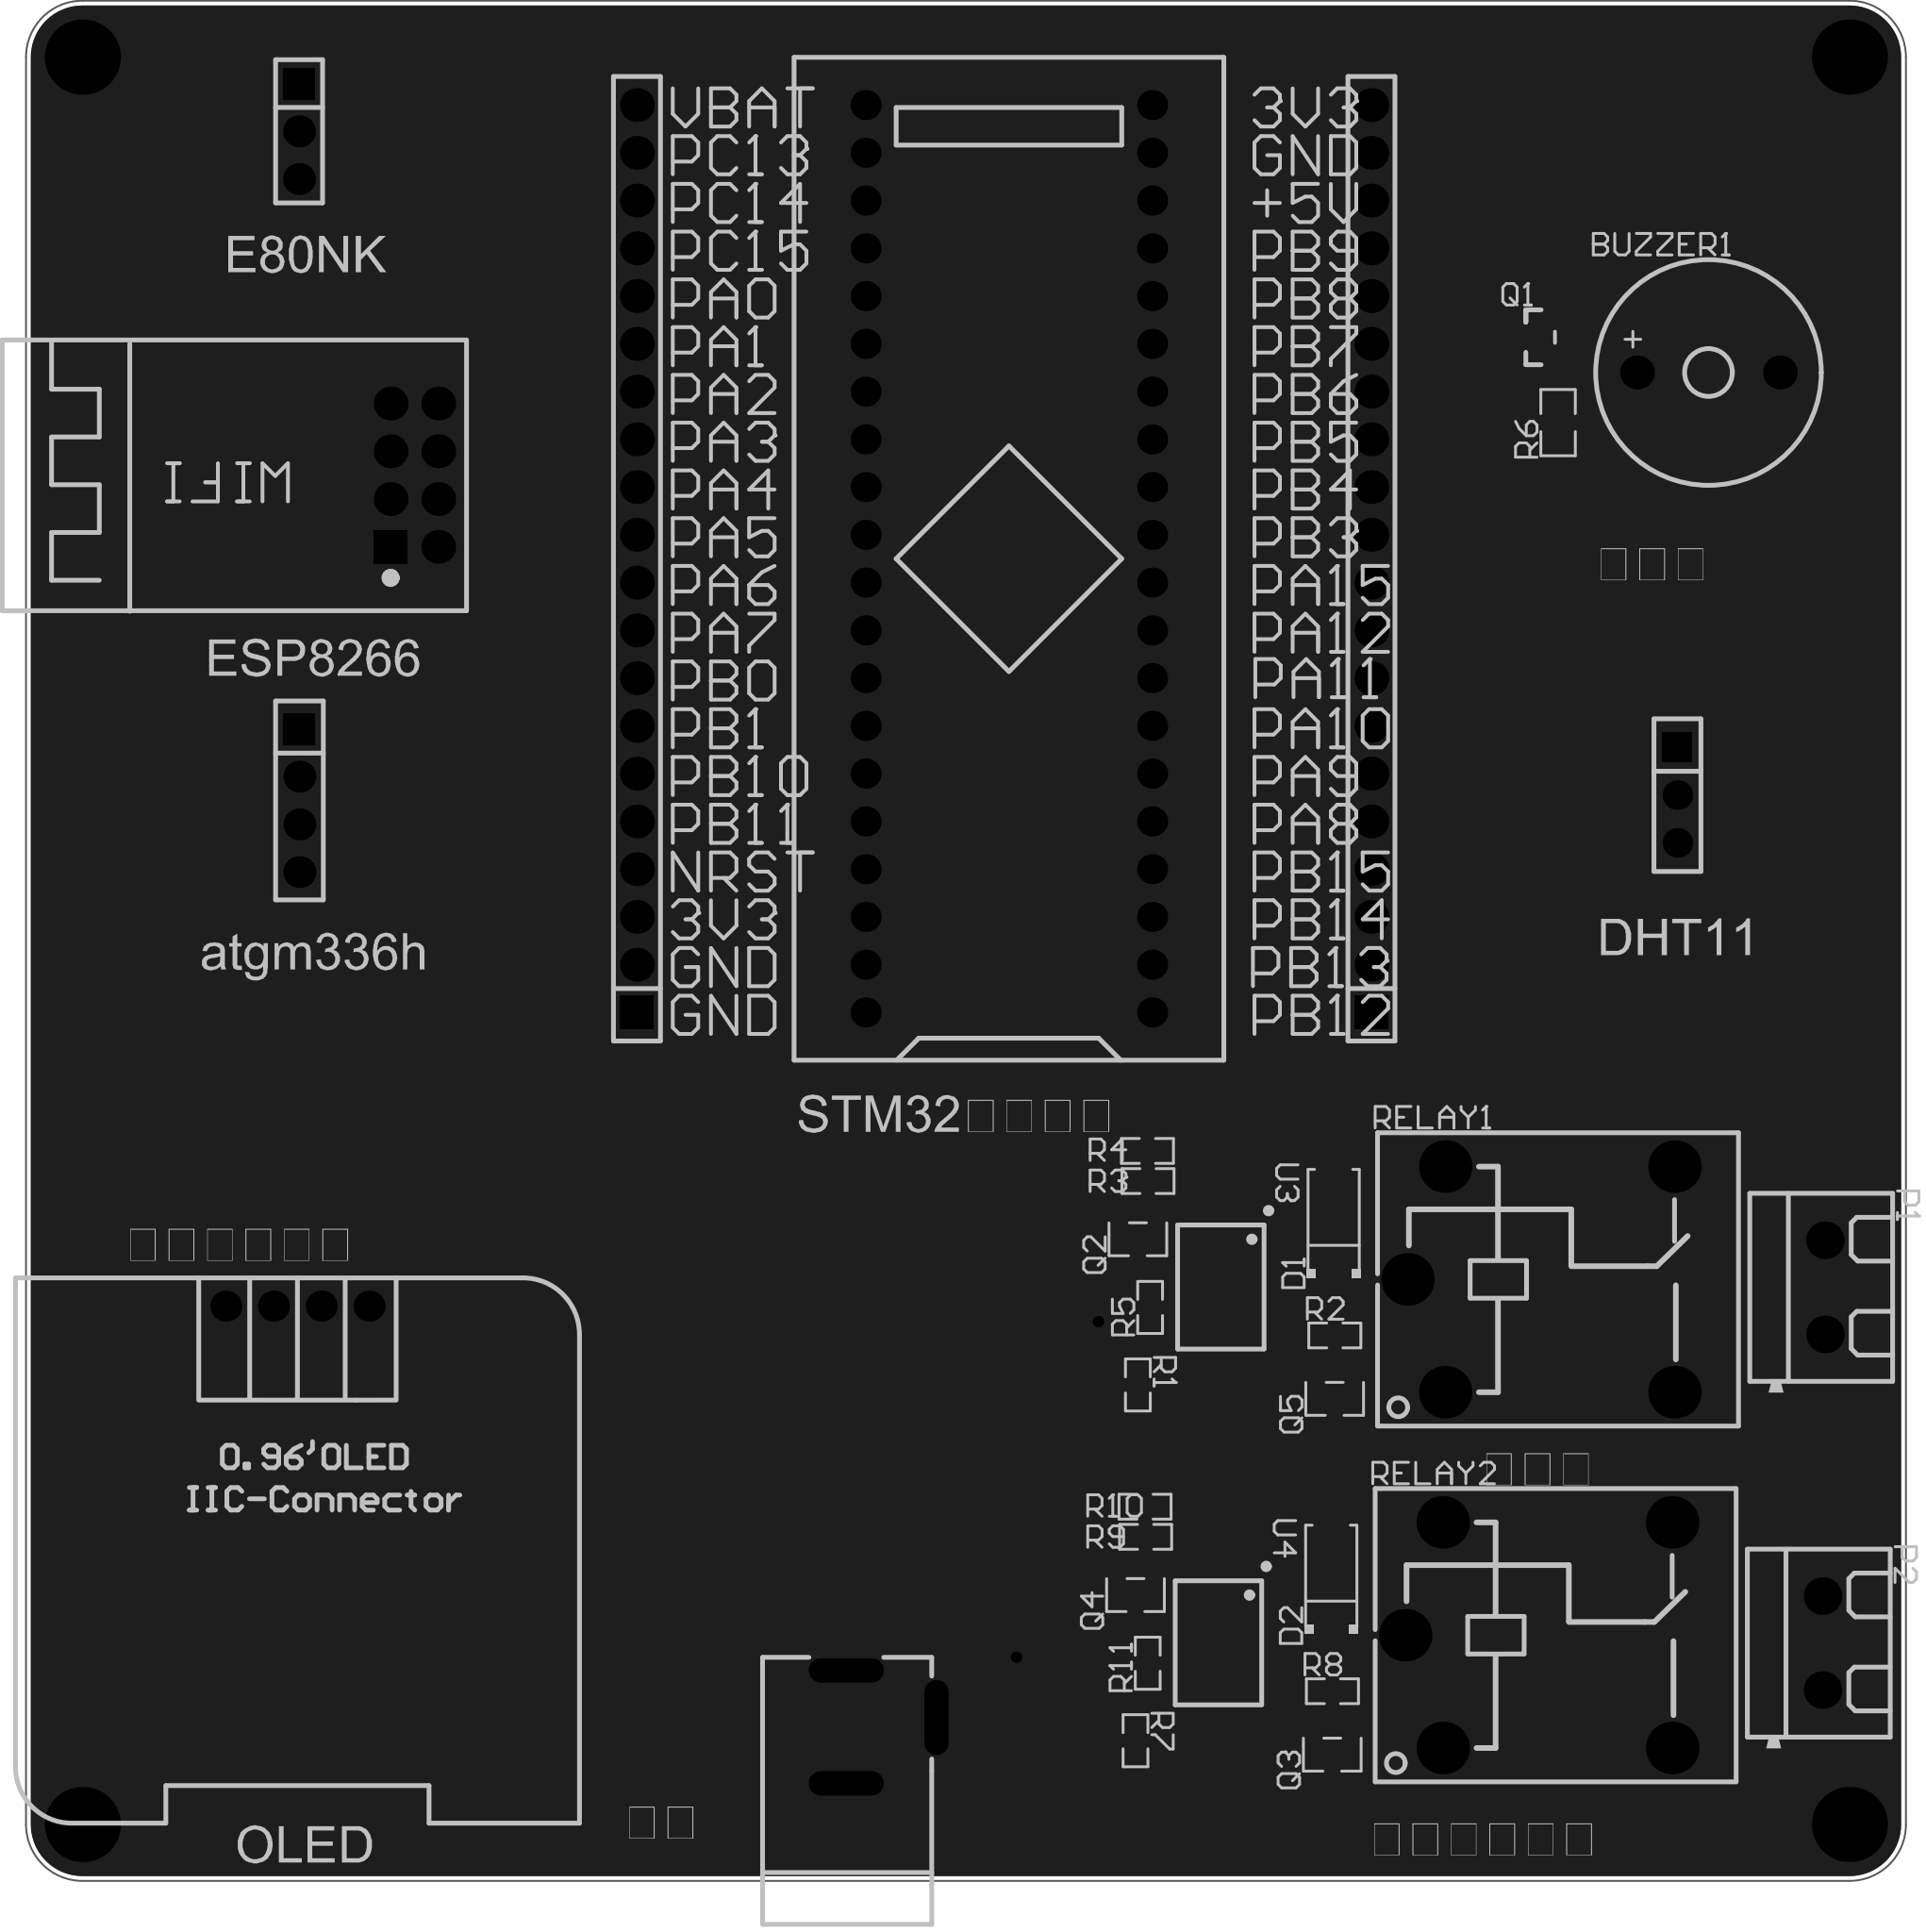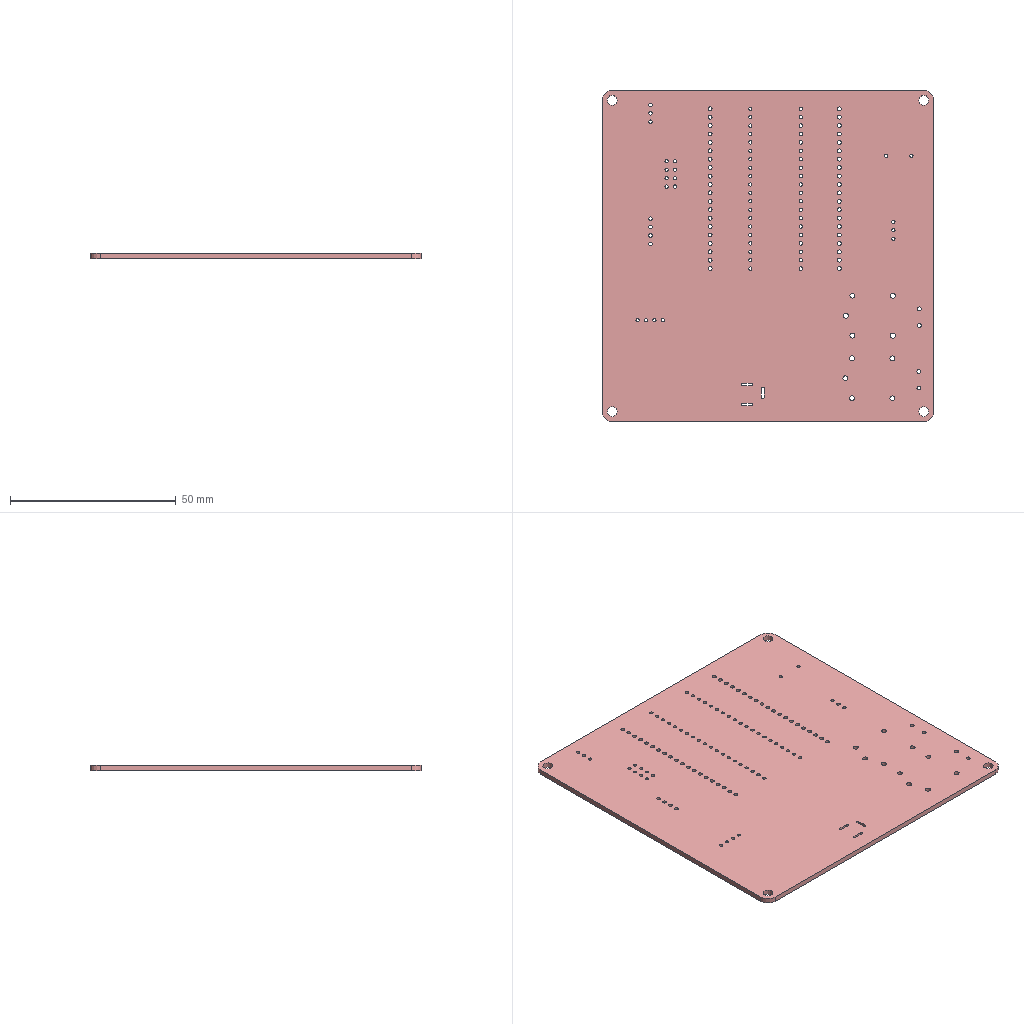Circuit board layout | Altium Designer | box 100 x 100 x 1.6 mm
Layer stack:
# Altium Designer layer stack of  (unit mm; dielectric type: 0 none, 1 core, 2 prepreg, 3 surface material)
index,name,kind,layer,copper_thickness_mm,dielectric_type,dielectric_thickness_mm,dielectric_material,dielectric_constant
0,Top Paste Mask Layer,other,,,,,,
1,Top Silkscreen Layer,other,,,,,,
2,Top Solder Mask Layer,dielectric,,,3,0.01,,3.3
3,Top Layer,copper,Top Layer,0.035,,,,
4,Dielectric1,dielectric,,,3,1.51,FR4,4.5
5,Bottom Layer,copper,Bottom Layer,0.035,,,,
6,Bottom Solder Mask Layer,dielectric,,,3,0.01,,3.3
7,Bottom Silkscreen Layer,other,,,,,,
8,Bottom Paste Mask Layer,other,,,,,,
# drill layer pairs: low layer,high layer
drill_pair,Top Layer,Bottom Layer
Part placement:
Designator,Comment,Layer,Footprint,Center-X(mm),Center-Y(mm),Rotation
U1,STM32F103C8T6-Card,TopLayer,CONN-TH_L53.3-W22.9_STM32F103C8T6-CARD,132.842,149.225,90
H1,,TopLayer,HDR-TH_20P-P2.54-V-F,152.125,149.225,90
H2,,TopLayer,HDR-TH_20P-P2.54-V-F,113.054,149.225,90
DC1,,TopLayer,DC-2.0,126.588,87.094,270
H5,,TopLayer,HDR-TH_3P-P2.54-V-F,168.402,136.652,270
H8,,TopLayer,HDR-TH_3P-P2.54-V-M,95.081,171.958,270
H6,,TopLayer,HDR-TH_4P-P2.54-V-F,95.101,136.37,270
OLED1,,TopLayer,0.96OLED_4P,94.996,109.474,0
U2,Ai-Thinker ESP-01S ESP8266,TopLayer,WIFIM-TH_8P-L24.7-W14.4-P2.54,101.219,153.67,180
BUZZER1,buzzer-12X9,TopLayer,BUZ-TH_BD12.0-P7.60-D0.6-FD,170.053,159.131,0
D1,US1M,TopLayer,SMA_L4.4-W2.8-LS5.4-RD,150.114,114.046,90
D2,US1M,TopLayer,SMA_L4.4-W2.8-LS5.4-RD,149.987,95.123,90
P1,KF301-2P接线端子,TopLayer,CONN-TH_XY301V-A-5.0-2P,176.249,110.474,270
P2,KF301-2P接线端子,TopLayer,CONN-TH_XY301V-A-5.0-2P,176.122,91.551,270
Q1,2N3906S-RTK/PS,TopLayer,SOT-23-3_L2.9-W1.3-P1.90-LS2.4-TR,160.987,161.004,0
Q2,S8050,TopLayer,SOT-23-3_L2.9-W1.6-P1.90-LS2.8-BR,139.7,113.03,90
Q3,S8050,TopLayer,SOT-23-3_L2.9-W1.6-P1.90-LS2.8-BR,150.041,85.62,90
Q4,S8050,TopLayer,SOT-23-3_L2.9-W1.6-P1.90-LS2.8-BR,139.573,94.107,90
Q5,S8050,TopLayer,SOT-23-3_L2.9-W1.6-P1.90-LS2.8-BR,150.168,104.543,90
R1,1kΩ,TopLayer,R0603,139.7,105.283,270
R2,10kΩ,TopLayer,R0603,150.177,107.915,0
R3,1kΩ,TopLayer,R0603,140.239,116.127,0
R4,10kΩ,TopLayer,R0603,140.208,117.729,0
R5,1kΩ,TopLayer,R0603,140.351,109.404,90
R6,2.2K,TopLayer,R0805,162.052,156.464,90
R7,1kΩ,TopLayer,R0603,139.573,86.36,270
R8,10kΩ,TopLayer,R0603,150.049,88.992,0
R9,1kΩ,TopLayer,R0603,140.112,97.204,0
R10,10kΩ,TopLayer,R0603,140.081,98.806,0
R11,1kΩ,TopLayer,R0603,140.224,90.481,90
RELAY1,SRD-12VDC-SL-C,TopLayer,RELAY-TH_SRD-XXVDC-XL-C,161.149,110.895,0
RELAY2,SRD-12VDC-SL-C,TopLayer,RELAY-TH_SRD-XXVDC-XL-C,161.022,91.972,0
U3,PC817C,TopLayer,OPTO-SMD-4_L4.6-W6.5-P2.54-LS10.3-TL,144.113,110.49,270
U4,PC817C,TopLayer,OPTO-SMD-4_L4.6-W6.5-P2.54-LS10.3-TL,143.986,91.567,270
Pad and via stacks:
# Altium Designer via and pad stacks of  (unit mm). Each distinct definition once, with the count of objects using it.
# via: kind,start_layer,end_layer,hole_mm,diameter_mm,mode(0 simple;1 top-mid-bottom;2 full stack),diameter_per_layer,count,example_net
# pad: kind,layer,hole_mm,hole_type(0 round;1 square;2 slot),plating,top_size,top_shape(1 round;2 rect;3 octagon;9 rounded rect),mid_size,bottom_size,mode,footprint,size_per_layer,count,example
pad,Multi-Layer,3,0,plated,4x4,1,4x4,4x4,0,,,4,1
pad,Multi-Layer,1,0,plated,1.6x1.6,1,1.6x1.6,1.6x1.6,0,CONN-TH_L53.3-W22.9_STM32F103C8T6-CARD,,40,U1.1
pad,Multi-Layer,1.2,0,plated,1.8x1.8,2,1.8x1.8,1.8x1.8,0,HDR-TH_20P-P2.54-V-F,,2,H1.1
pad,Multi-Layer,1.2,0,plated,1.8x1.8,1,1.8x1.8,1.8x1.8,0,HDR-TH_20P-P2.54-V-F,,38,H1.2
pad,Multi-Layer,0.8001,2,plated,4x1.3,1,4x1.3,4x1.3,0,DC-2.0,,3,DC1.2
pad,Multi-Layer,1.02,0,plated,1.575x1.575,1,1.575x1.575,1.575x1.575,0,HDR-TH_3P-P2.54-V-F,,2,H5.3
pad,Multi-Layer,1.02,0,plated,1.575x1.575,2,1.575x1.575,1.575x1.575,0,HDR-TH_3P-P2.54-V-F,,1,H5.1
pad,Multi-Layer,1.1,0,plated,1.7x1.7,2,1.7x1.7,1.7x1.7,0,HDR-TH_3P-P2.54-V-M,,1,H8.1
pad,Multi-Layer,1.1,0,plated,1.7x1.7,1,1.7x1.7,1.7x1.7,0,HDR-TH_3P-P2.54-V-M,,2,H8.2
pad,Multi-Layer,1.1,0,plated,1.7x1.7,2,1.7x1.7,1.7x1.7,0,HDR-TH_4P-P2.54-V-F,,1,H6.1
pad,Multi-Layer,1.1,0,plated,1.7x1.7,1,1.7x1.7,1.7x1.7,0,HDR-TH_4P-P2.54-V-F,,3,H6.2
pad,Multi-Layer,1,0,plated,1.65x1.65,1,1.65x1.65,1.65x1.65,0,0.96OLED_4P,,4,OLED1.4
pad,Multi-Layer,1,0,plated,1.8x1.8,1,1.8x1.8,1.8x1.8,0,WIFIM-TH_8P-L24.7-W14.4-P2.54,,7,U2.8
pad,Multi-Layer,1,0,plated,1.8x1.8,2,1.8x1.8,1.8x1.8,0,WIFIM-TH_8P-L24.7-W14.4-P2.54,,1,U2.1
pad,Multi-Layer,1,0,plated,1.8x1.8,1,1.8x1.8,1.8x1.8,0,BUZ-TH_BD12.0-P7.60-D0.6-FD,,2,BUZZER1.2
pad,Multi-Layer,1.2,0,plated,2x2,1,2x2,2x2,0,CONN-TH_XY301V-A-5.0-2P,,4,P1.1
pad,Multi-Layer,1.524,0,plated,2.794x2.794,1,2.794x2.794,2.794x2.794,0,RELAY-TH_SRD-XXVDC-XL-C,,10,RELAY1.2
pad,Top Layer,0,0,plated,2.046x1.62,2,2.046x1.62,2.046x1.62,0,SMA_L4.4-W2.8-LS5.4-RD,,4,D1.2
pad,Top Layer,0,0,plated,0.7x1.25,2,0.7x1.25,0.7x1.25,0,SOT-23-3_L2.9-W1.3-P1.90-LS2.4-TR,,3,Q1.3
pad,Top Layer,0,0,plated,1.07x0.6,2,1.07x0.6,1.07x0.6,0,SOT-23-3_L2.9-W1.6-P1.90-LS2.8-BR,,12,Q2.1
pad,Top Layer,0,0,plated,0.8065x0.864,2,0.8065x0.864,0.8065x0.864,0,R0603,,20,R1.2
pad,Top Layer,0,0,plated,1.133x1.377,2,1.133x1.377,1.133x1.377,0,R0805,,2,R6.2
pad,Top Layer,0,0,plated,1.5x3,2,1.5x3,1.5x3,0,OPTO-SMD-4_L4.6-W6.5-P2.54-LS10.3-TL,,8,U3.4
via,Top Layer,Bottom Layer,0.3048,0.61,0,,2,+5V
Copper pours:
name,layer,net,type(0 solid;1 hatched;2 none)
Bottom Layer-GND,Bottom Layer,GND,0
Top Layer-GND,Top Layer,GND,0